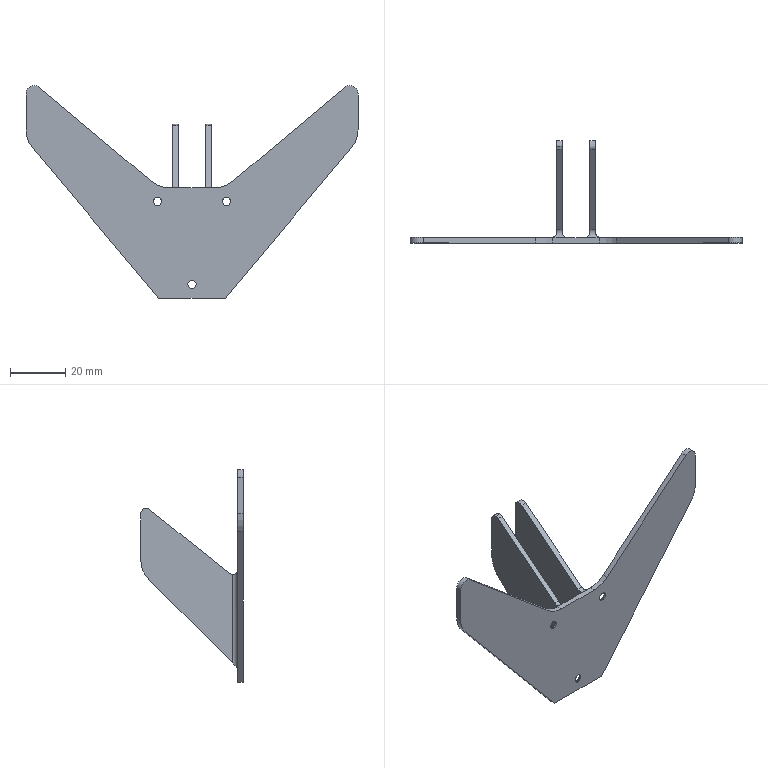Part | SolidWorks | features BaseBody 1 | 1 solid | 52 faces | box 120 x 37 x 76.843 mm | volume 11950 mm3 | cylinder 25 | plane 21 | cone 6 | commonest cylinder face diameters 4 x11 3 x6 20 x6 6 x2